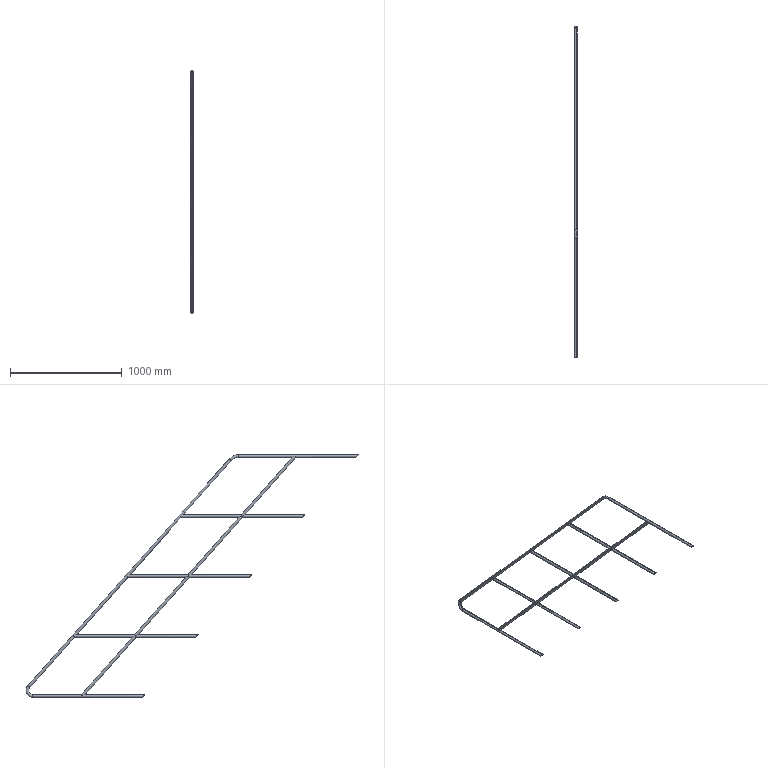Part | STEP file | 粉仓楼梯护栏主体_Default<As Machined> | 12 solids | 80 faces | box 25 x 2968 x 2169 mm | volume 1217350 mm3 | cylinder 59 | plane 13 | torus 8 | commonest cylinder face diameters 25 x39 22 x20